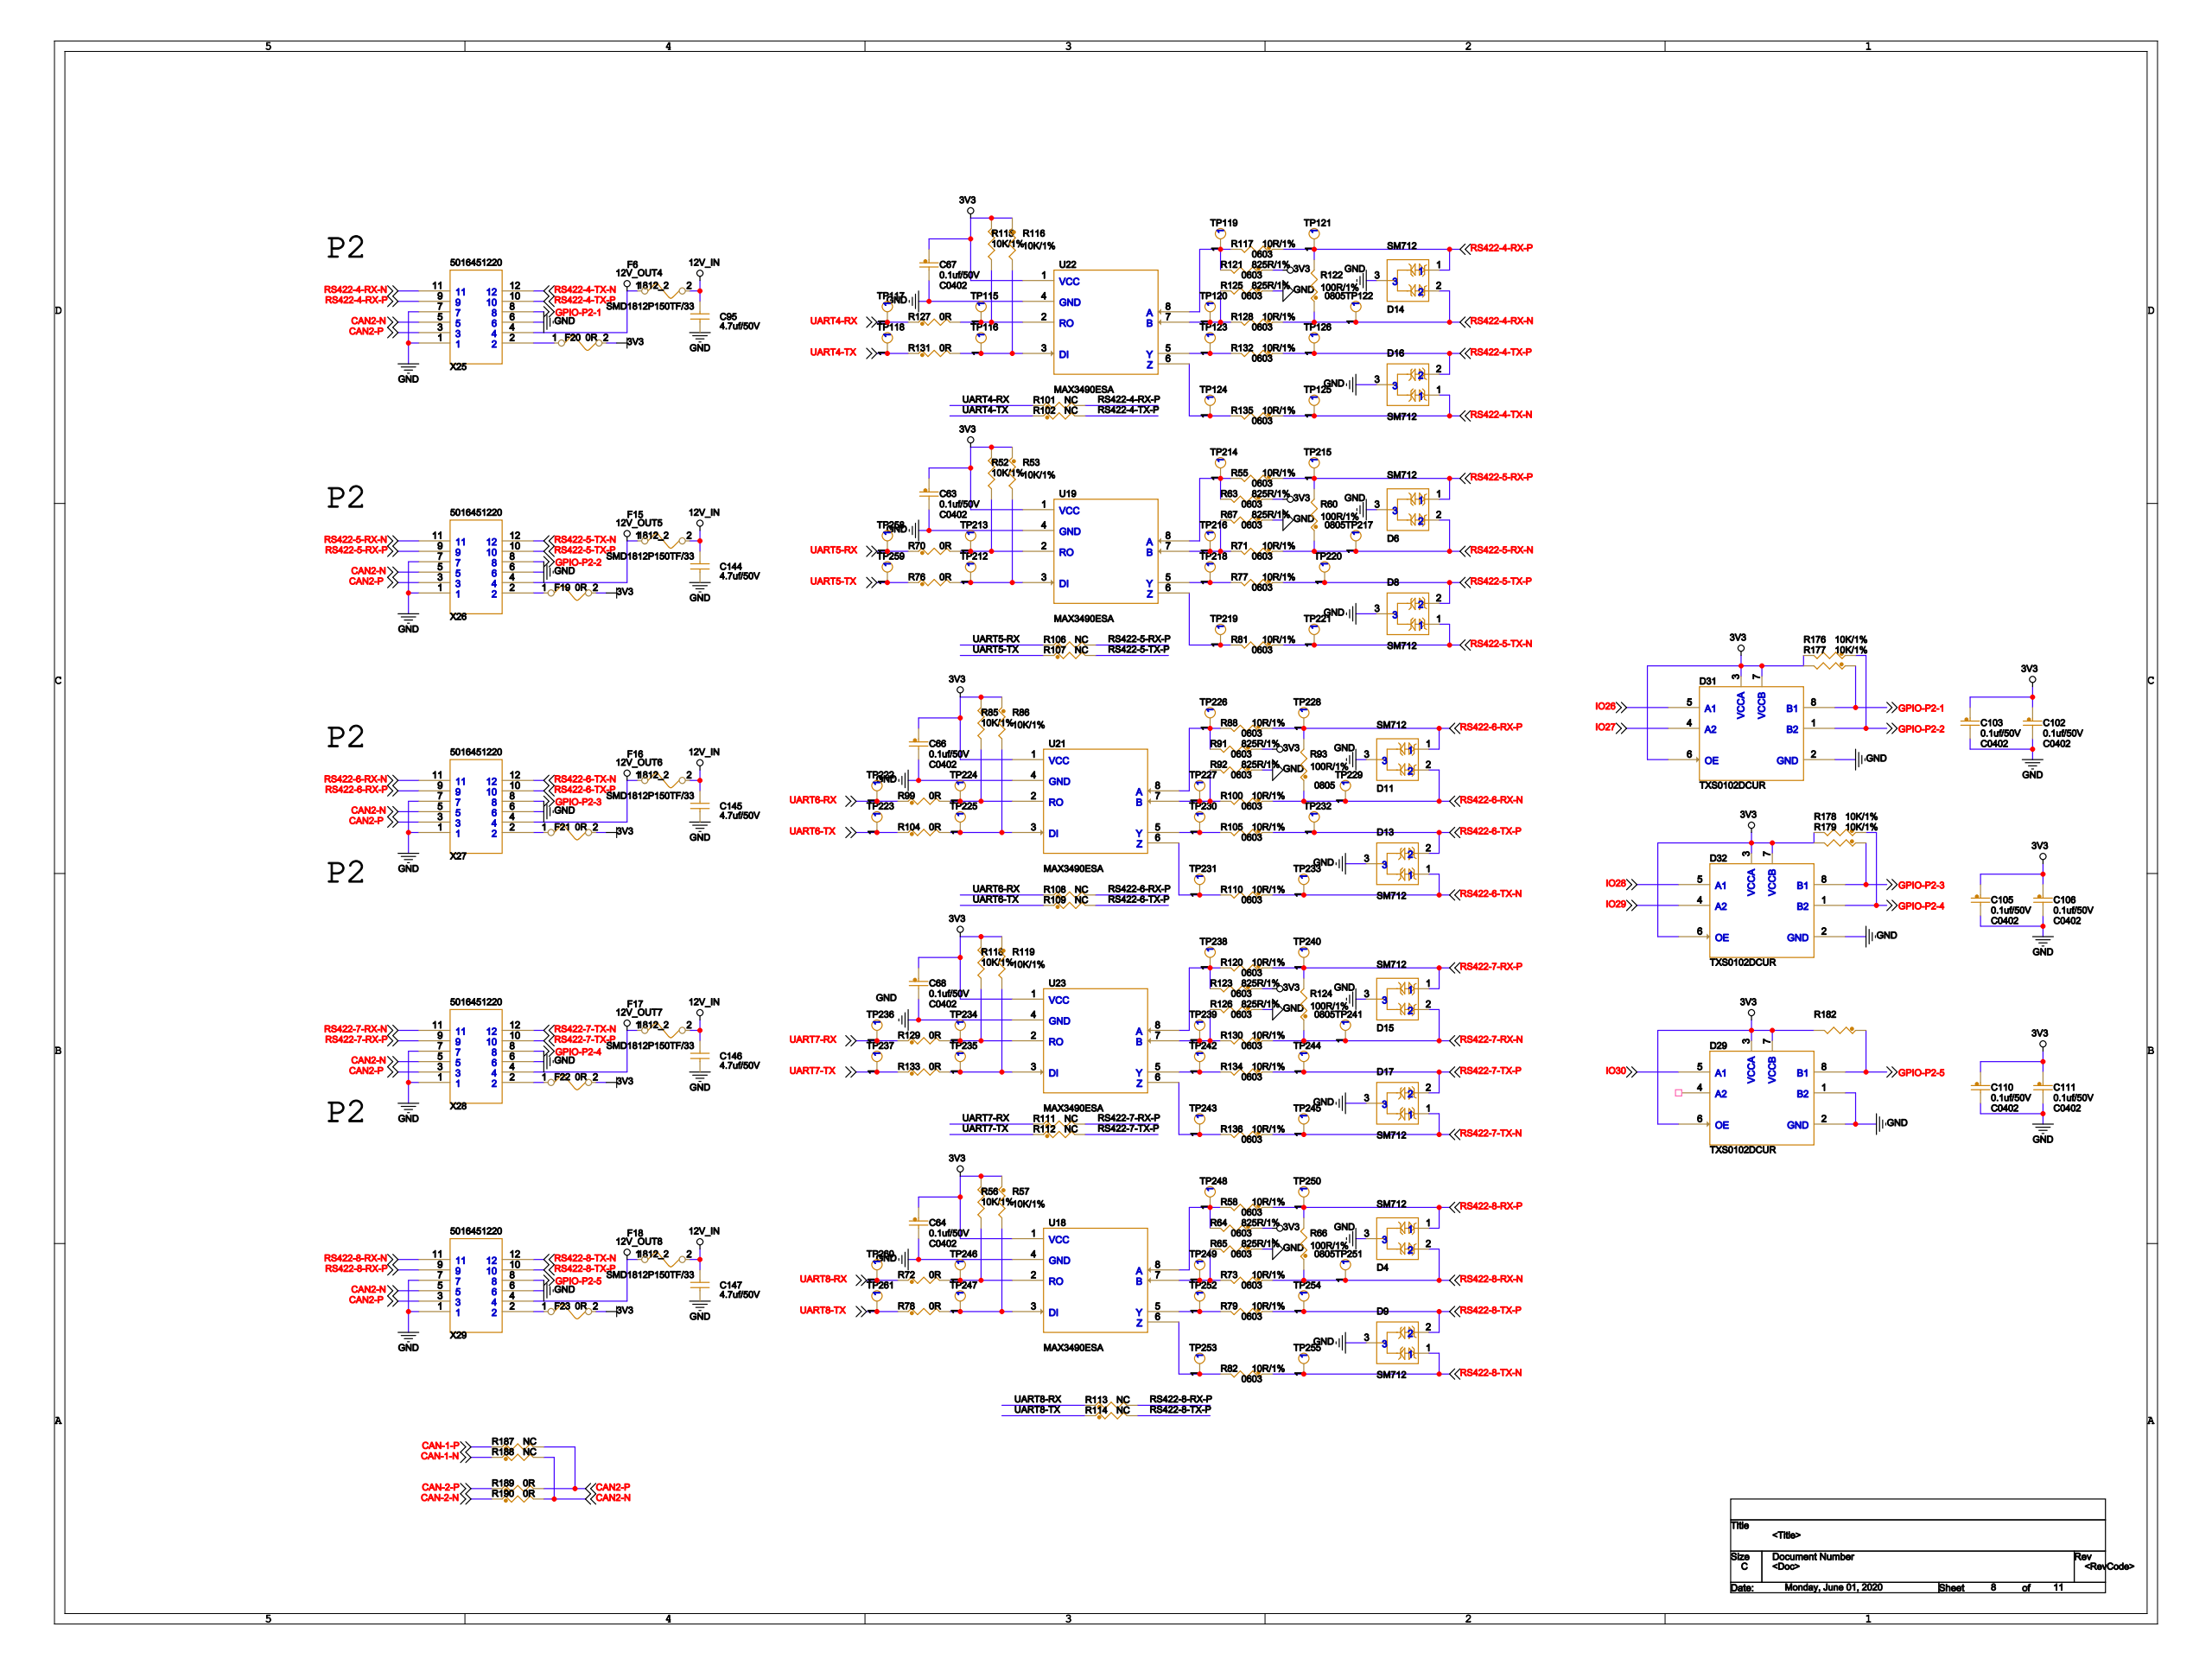Circuit board | Cadence Allegro | 792 parts | 400 nets | one sheet of the schematic
Parts on this sheet (reference | value | footprint):
C63 | 0.1uf/50V | C0402
C64 | 0.1uf/50V | C0402
C66 | 0.1uf/50V | C0402
C67 | 0.1uf/50V | C0402
C68 | 0.1uf/50V | C0402
C95 | 4.7uf/50V | C0805
C102 | 0.1uf/50V | C0402
C103 | 0.1uf/50V | C0402
C105 | 0.1uf/50V | C0402
C106 | 0.1uf/50V | C0402
C110 | 0.1uf/50V | C0402
C111 | 0.1uf/50V | C0402
C144 | 4.7uf/50V | C0805
C145 | 4.7uf/50V | C0805
C146 | 4.7uf/50V | C0805
C147 | 4.7uf/50V | C0805
D4 | SM712 | SOT23
D6 | SM712 | SOT23
D8 | SM712 | SOT23
D9 | SM712 | SOT23
D11 | SM712 | SOT23
D13 | SM712 | SOT23
D14 | SM712 | SOT23
D15 | SM712 | SOT23
D16 | SM712 | SOT23
D17 | SM712 | SOT23
D29 | TXS0102DCUR | VSSOP8
D31 | TXS0102DCUR | VSSOP8
D32 | TXS0102DCUR | VSSOP8
F6 | SMD1812P150TF/33 | 1812_2
F15 | SMD1812P150TF/33 | 1812_2
F16 | SMD1812P150TF/33 | 1812_2
F17 | SMD1812P150TF/33 | 1812_2
F18 | SMD1812P150TF/33 | 1812_2
F19 | 0R | 0603
F20 | 0R | 0603
F21 | 0R | 0603
F22 | 0R | 0603
F23 | 0R | 0603
R52 | 10K/1% | 0402
R53 | 10K/1% | 0402
R55 | 10R/1% | 0603
R56 | 10K/1% | 0402
R57 | 10K/1% | 0402
R58 | 10R/1% | 0603
R60 | 100R/1% | 0805
R63 | 825R/1% | 0603
R64 | 825R/1% | 0603
R65 | 825R/1% | 0603
R66 | 100R/1% | 0805
R67 | 825R/1% | 0603
R70 | 0R | 0603
R71 | 10R/1% | 0603
R72 | 0R | 0603
R73 | 10R/1% | 0603
R76 | 0R | 0603
R77 | 10R/1% | 0603
R78 | 0R | 0603
R79 | 10R/1% | 0603
R81 | 10R/1% | 0603
R82 | 10R/1% | 0603
R85 | 10K/1% | 0402
R86 | 10K/1% | 0402
R88 | 10R/1% | 0603
R91 | 825R/1% | 0603
R92 | 825R/1% | 0603
R93 | 100R/1% | 0805
R99 | 0R | 0603
R100 | 10R/1% | 0603
R101 | NC | 0603
R102 | NC | 0603
R104 | 0R | 0603
R105 | 10R/1% | 0603
R106 | NC | 0603
R107 | NC | 0603
R108 | NC | 0603
R109 | NC | 0603
R110 | 10R/1% | 0603
R111 | NC | 0603
R112 | NC | 0603
R113 | NC | 0603
R114 | NC | 0603
R115 | 10K/1% | 0402
R116 | 10K/1% | 0402
R117 | 10R/1% | 0603
R118 | 10K/1% | 0402
R119 | 10K/1% | 0402
R120 | 10R/1% | 0603
R121 | 825R/1% | 0603
R122 | 100R/1% | 0805
R123 | 825R/1% | 0603
R124 | 100R/1% | 0805
R125 | 825R/1% | 0603
R126 | 825R/1% | 0603
R127 | 0R | 0603
R128 | 10R/1% | 0603
R129 | 0R | 0603
R130 | 10R/1% | 0603
R131 | 0R | 0603
R132 | 10R/1% | 0603
R133 | 0R | 0603
R134 | 10R/1% | 0603
R135 | 10R/1% | 0603
R136 | 10R/1% | 0603
R176 | 10K/1% | 0402
R177 | 10K/1% | 0402
R178 | 10K/1% | 0402
R179 | 10K/1% | 0402
R182 | 10K/1% | 0402
R187 | NC | 0603
R188 | NC | 0603
R189 | 0R | 0603
R190 | 0R | 0603
TP115 | TESTPOINT | TESTPOINT-33MIL
TP116 | TESTPOINT | TESTPOINT-33MIL
TP117 | TESTPOINT | TESTPOINT-33MIL
TP118 | TESTPOINT | TESTPOINT-33MIL
TP119 | TESTPOINT | TESTPOINT-33MIL
TP120 | TESTPOINT | TESTPOINT-33MIL
TP121 | TESTPOINT | TESTPOINT-33MIL
TP122 | TESTPOINT | TESTPOINT-33MIL
TP123 | TESTPOINT | TESTPOINT-33MIL
TP124 | TESTPOINT | TESTPOINT-33MIL
TP125 | TESTPOINT | TESTPOINT-33MIL
TP126 | TESTPOINT | TESTPOINT-33MIL
TP212 | TESTPOINT | TESTPOINT-33MIL
TP213 | TESTPOINT | TESTPOINT-33MIL
TP214 | TESTPOINT | TESTPOINT-33MIL
TP215 | TESTPOINT | TESTPOINT-33MIL
TP216 | TESTPOINT | TESTPOINT-33MIL
TP217 | TESTPOINT | TESTPOINT-33MIL
TP218 | TESTPOINT | TESTPOINT-33MIL
TP219 | TESTPOINT | TESTPOINT-33MIL
TP220 | TESTPOINT | TESTPOINT-33MIL
TP221 | TESTPOINT | TESTPOINT-33MIL
TP222 | TESTPOINT | TESTPOINT-33MIL
TP223 | TESTPOINT | TESTPOINT-33MIL
TP224 | TESTPOINT | TESTPOINT-33MIL
TP225 | TESTPOINT | TESTPOINT-33MIL
TP226 | TESTPOINT | TESTPOINT-33MIL
TP227 | TESTPOINT | TESTPOINT-33MIL
TP228 | TESTPOINT | TESTPOINT-33MIL
TP229 | TESTPOINT | TESTPOINT-33MIL
TP230 | TESTPOINT | TESTPOINT-33MIL
TP231 | TESTPOINT | TESTPOINT-33MIL
TP232 | TESTPOINT | TESTPOINT-33MIL
TP233 | TESTPOINT | TESTPOINT-33MIL
TP234 | TESTPOINT | TESTPOINT-33MIL
TP235 | TESTPOINT | TESTPOINT-33MIL
TP236 | TESTPOINT | TESTPOINT-33MIL
TP237 | TESTPOINT | TESTPOINT-33MIL
TP238 | TESTPOINT | TESTPOINT-33MIL
TP239 | TESTPOINT | TESTPOINT-33MIL
TP240 | TESTPOINT | TESTPOINT-33MIL
TP241 | TESTPOINT | TESTPOINT-33MIL
TP242 | TESTPOINT | TESTPOINT-33MIL
TP243 | TESTPOINT | TESTPOINT-33MIL
TP244 | TESTPOINT | TESTPOINT-33MIL
TP245 | TESTPOINT | TESTPOINT-33MIL
TP246 | TESTPOINT | TESTPOINT-33MIL
TP247 | TESTPOINT | TESTPOINT-33MIL
TP248 | TESTPOINT | TESTPOINT-33MIL
TP249 | TESTPOINT | TESTPOINT-33MIL
TP250 | TESTPOINT | TESTPOINT-33MIL
TP251 | TESTPOINT | TESTPOINT-33MIL
TP252 | TESTPOINT | TESTPOINT-33MIL
TP253 | TESTPOINT | TESTPOINT-33MIL
TP254 | TESTPOINT | TESTPOINT-33MIL
TP255 | TESTPOINT | TESTPOINT-33MIL
TP258 | TESTPOINT | TESTPOINT-33MIL
TP259 | TESTPOINT | TESTPOINT-33MIL
TP260 | TESTPOINT | TESTPOINT-33MIL
TP261 | TESTPOINT | TESTPOINT-33MIL
U18 | MAX3490ESA | SOP8
U19 | MAX3490ESA | SOP8
U21 | MAX3490ESA | SOP8
U22 | MAX3490ESA | SOP8
U23 | MAX3490ESA | SOP8
X25 | 5016451220 | 5016451220
X26 | 5016451220 | 5016451220
X27 | 5016451220 | 5016451220
X28 | 5016451220 | 5016451220
X29 | 5016451220 | 5016451220
Nets of these parts (net: part-pin ...):
N8121676: F19-1 X26-2
3V3: C63-1 C64-1 C66-1 C67-1 C68-1 C102-1 C103-1 C105-1 C106-1 C110-1 C111-1 D29-3 D29-6 D29-7 D31-3 D31-6 D31-7 D32-3 D32-6 D32-7 F19-2 F20-2 F21-2 F22-2 F23-2 R52-1 R53-1 R56-1 R57-1 R63-1 R64-1 R85-1 R86-1 R91-1 R115-1 R116-1 R118-1 R119-1 R121-1 R123-1 R176-2 R177-2 R178-2 R179-2 R182-2 U18-1 U19-1 U21-1 U22-1 U23-1
N8084713: F20-1 X25-2
N8122407: F21-1 X27-2
N8122712: F22-1 X28-2
N8123018: F23-1 X29-2
GND: C63-2 C64-2 C66-2 C67-2 C68-2 C95-2 C102-2 C103-2 C105-2 C106-2 C110-2 C111-2 C144-2 C145-2 C146-2 C147-2 D4-3 D6-3 D8-3 D9-3 D11-3 D13-3 D14-3 D15-3 D16-3 D17-3 D29-1 D29-2 D31-2 D32-2 R65-1 R67-1 R92-1 R125-1 R126-1 U18-4 U19-4 U21-4 U22-4 U23-4 X25-1 X25-6 X25-7 X26-1 X26-6 X26-7 X27-1 X27-6 X27-7 X28-1 X28-6 X28-7 X29-1 X29-6 X29-7
RS422-4-TX-P: D16-2 R102-2 R132-1 TP126-1 X25-10
RS422-4-RX-N: D14-2 R122-1 R128-1 TP122-1 X25-11
RS422-4-TX-N: D16-1 R135-1 TP125-1 X25-12
CAN2-P: R187-2 R189-2 X25-3 X26-3 X27-3 X28-3 X29-3
12V_OUT4: F6-1 X25-4
CAN2-N: R188-2 R190-2 X25-5 X26-5 X27-5 X28-5 X29-5
GPIO-P2-1: D31-8 R177-1 X25-8
RS422-4-RX-P: D14-1 R101-2 R117-1 R122-2 TP121-1 X25-9
RS422-5-TX-P: D8-2 R77-1 R107-2 TP220-1 X26-10
RS422-5-RX-N: D6-2 R60-1 R71-1 TP217-1 X26-11
RS422-5-TX-N: D8-1 R81-1 TP221-1 X26-12
12V_OUT5: F15-1 X26-4
GPIO-P2-2: D31-1 R176-1 X26-8
RS422-5-RX-P: D6-1 R55-1 R60-2 R106-2 TP215-1 X26-9
RS422-6-TX-P: D13-2 R105-1 R109-2 TP232-1 X27-10
RS422-6-RX-N: D11-2 R93-1 R100-1 TP229-1 X27-11
RS422-6-TX-N: D13-1 R110-1 TP233-1 X27-12
12V_OUT6: F16-1 X27-4
GPIO-P2-3: D32-8 R179-1 X27-8
RS422-6-RX-P: D11-1 R88-1 R93-2 R108-2 TP228-1 X27-9
RS422-7-TX-P: D17-2 R112-2 R134-1 TP244-1 X28-10
RS422-7-RX-N: D15-2 R124-1 R130-1 TP241-1 X28-11
RS422-7-TX-N: D17-1 R136-1 TP245-1 X28-12
12V_OUT7: F17-1 X28-4
GPIO-P2-4: D32-1 R178-1 X28-8
RS422-7-RX-P: D15-1 R111-2 R120-1 R124-2 TP240-1 X28-9
RS422-8-TX-P: D9-2 R79-1 R114-2 TP254-1 X29-10
RS422-8-RX-N: D4-2 R66-1 R73-1 TP251-1 X29-11
RS422-8-TX-N: D9-1 R82-1 TP255-1 X29-12
12V_OUT8: F18-1 X29-4
GPIO-P2-5: D29-8 R182-1 X29-8
RS422-8-RX-P: D4-1 R58-1 R66-2 R113-2 TP250-1 X29-9
CAN-1-P: R187-1
CAN-1-N: R188-1
12V_IN: C95-1 C144-1 C145-1 C146-1 C147-1 F6-2 F15-2 F16-2 F17-2 F18-2
UART5-RX: R70-1 R106-1 TP258-1
UART5-TX: R76-1 R107-1 TP259-1
UART8-RX: R72-1 R113-1 TP260-1
UART8-TX: R78-1 R114-1 TP261-1
N8056583: R53-2 R76-2 TP212-1 U19-3
N8056575: R52-2 R70-2 TP213-1 U19-2
N8056105: R55-2 R63-2 TP214-1 U19-8
N8056413: R67-2 R71-2 TP216-1 U19-7
N8056379: R77-2 TP218-1 U19-5
N8056117: R81-2 TP219-1 U19-6
UART6-RX: R99-1 R108-1 TP222-1
UART6-TX: R104-1 R109-1 TP223-1
N8058346: R85-2 R99-2 TP224-1 U21-2
N8058354: R86-2 R104-2 TP225-1 U21-3
N8057884: R88-2 R91-2 TP226-1 U21-8
N8058184: R92-2 R100-2 TP227-1 U21-7
N8058150: R105-2 TP230-1 U21-5
N8057888: R110-2 TP231-1 U21-6
N8060155: R118-2 R129-2 TP234-1 U23-2
N8060163: R119-2 R133-2 TP235-1 U23-3
UART7-RX: R111-1 R129-1 TP236-1
UART7-TX: R112-1 R133-1 TP237-1
N8059693: R120-2 R123-2 TP238-1 U23-8
N8059993: R126-2 R130-2 TP239-1 U23-7
N8059935: R134-2 TP242-1 U23-5
N8059697: R136-2 TP243-1 U23-6
N8061600: R56-2 R72-2 TP246-1 U18-2
N8061608: R57-2 R78-2 TP247-1 U18-3
N8061616: R58-2 R64-2 TP248-1 U18-8
N8061916: R65-2 R73-2 TP249-1 U18-7
N8061882: R79-2 TP252-1 U18-5
N8061620: R82-2 TP253-1 U18-6
N8053150: R115-2 R127-2 TP115-1 U22-2
N8053158: R116-2 R131-2 TP116-1 U22-3
UART4-RX: R101-1 R127-1 TP117-1
UART4-TX: R102-1 R131-1 TP118-1
N8052964: R117-2 R121-2 TP119-1 U22-8
N8052972: R125-2 R128-2 TP120-1 U22-7
N8052938: R132-2 TP123-1 U22-5
N8052942: R135-2 TP124-1 U22-6
CAN-2-N: R190-1
CAN-2-P: R189-1
IO30: D29-5
IO26: D31-5
IO27: D31-4
IO28: D32-5
IO29: D32-4